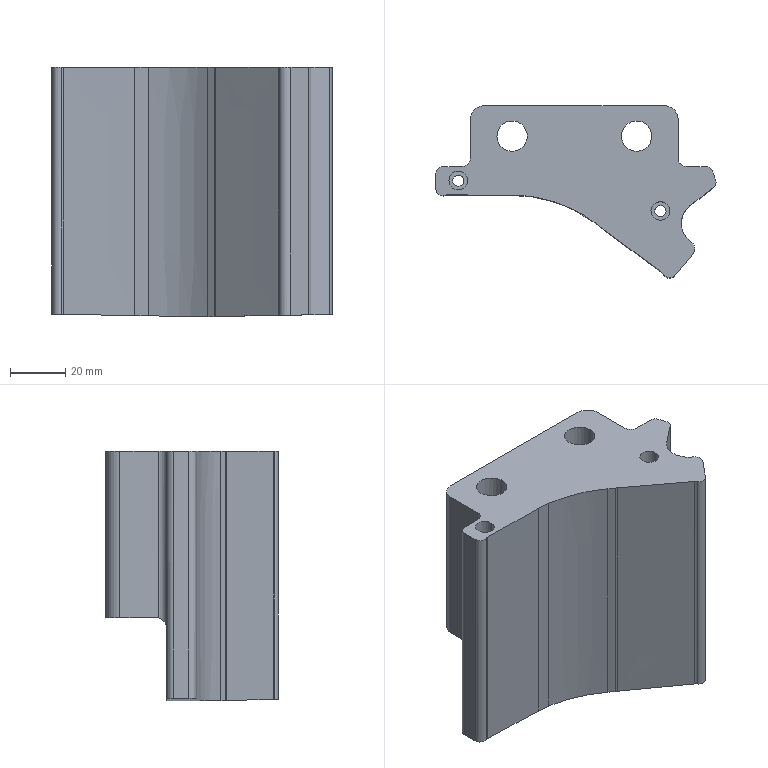Part | STEP file | gslz 2016.10.28-10_id3198_x_t | 1 solid | 46 faces | box 101.187 x 62.226 x 90 mm | volume 237811 mm3 | cylinder 23 | plane 20 | other 3 | commonest cylinder face diameters 5 x7 6 x3 4.1 x2 6.8 x2 10 x2 11 x2